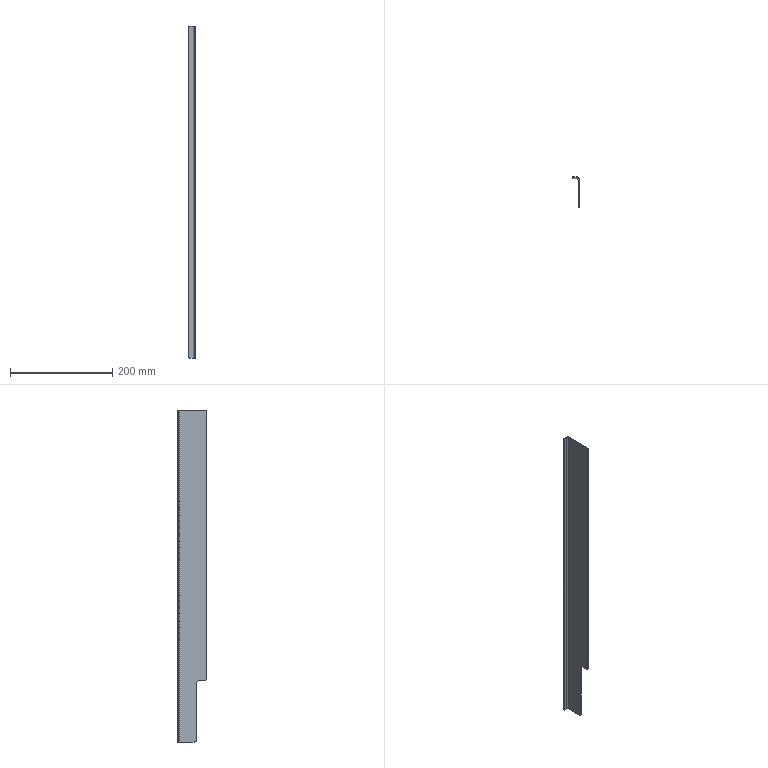Part | STEP file | 001-010-Waste sensor mounting seat | 1 solid | 22 faces | box 12 x 58 x 650 mm | volume 81910 mm3 | plane 14 | cylinder 8 | commonest cylinder face diameters 4 x4 10 x3 8 x1